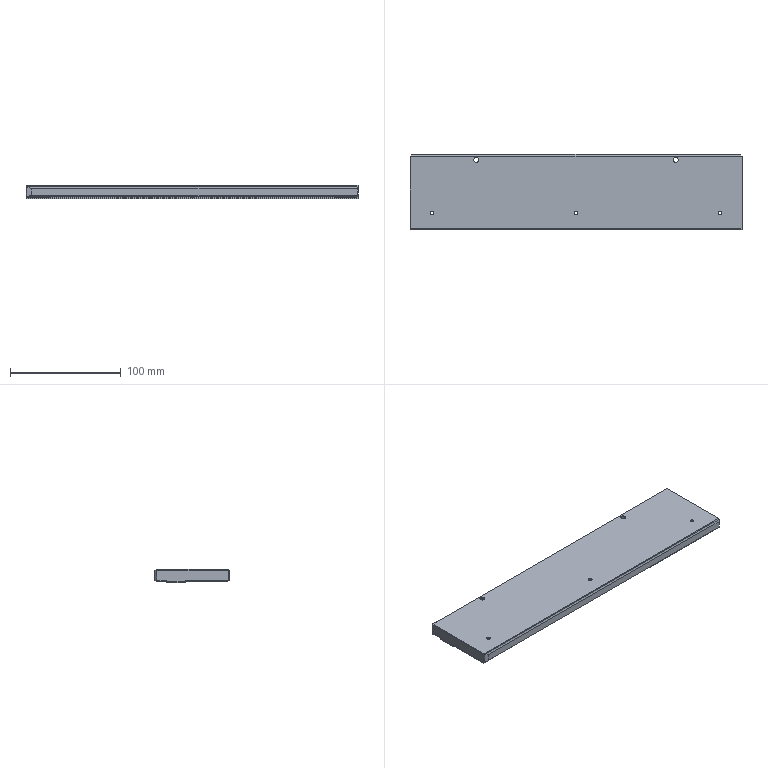Part | 2 solids | 48 faces | box 300 x 68 x 12 mm | volume 409266 mm3 | plane 38 | cylinder 10 | commonest cylinder face diameters 3.242 x6 4.5 x4
STEP:
#1=CARTESIAN_POINT('',(-150.,23.,-6.));
#2=VERTEX_POINT('',#1);
#3=CARTESIAN_POINT('',(150.,23.,-6.));
#4=VERTEX_POINT('',#3);
#5=CARTESIAN_POINT('',(-150.,23.,-6.));
#6=DIRECTION('',(1.,0.,0.));
#7=VECTOR('',#6,1000.);
#8=LINE('',#5,#7);
#9=EDGE_CURVE('',#2,#4,#8,.T.);
#10=ORIENTED_EDGE('',*,*,#9,.T.);
#11=CARTESIAN_POINT('',(150.,6.,-6.));
#12=VERTEX_POINT('',#11);
#13=CARTESIAN_POINT('',(150.,0.,-6.));
#14=DIRECTION('',(0.,-1.,0.));
#15=VECTOR('',#14,1000.);
#16=LINE('',#13,#15);
#17=EDGE_CURVE('',#4,#12,#16,.T.);
#18=ORIENTED_EDGE('',*,*,#17,.T.);
#19=CARTESIAN_POINT('',(-150.,6.,-6.));
#20=VERTEX_POINT('',#19);
#21=CARTESIAN_POINT('',(150.,6.,-6.));
#22=DIRECTION('',(-1.,0.,0.));
#23=VECTOR('',#22,1000.);
#24=LINE('',#21,#23);
#25=EDGE_CURVE('',#12,#20,#24,.T.);
#26=ORIENTED_EDGE('',*,*,#25,.T.);
#27=CARTESIAN_POINT('',(-150.,0.,-6.));
#28=DIRECTION('',(0.,1.,0.));
#29=VECTOR('',#28,1000.);
#30=LINE('',#27,#29);
#31=EDGE_CURVE('',#20,#2,#30,.T.);
#32=ORIENTED_EDGE('',*,*,#31,.T.);
#33=EDGE_LOOP('',(#10,#18,#26,#32));
#34=FACE_BOUND('',#33,.T.);
#35=CARTESIAN_POINT('',(0.,0.,-6.));
#36=DIRECTION('',(0.,0.,-1.));
#37=DIRECTION('',(-1.,0.,0.));
#38=AXIS2_PLACEMENT_3D('',#35,#36,#37);
#39=PLANE('',#38);
#40=ADVANCED_FACE('',(#34),#39,.T.);
#41=CARTESIAN_POINT('',(92.25,29.,6.));
#42=VERTEX_POINT('',#41);
#43=CARTESIAN_POINT('',(90.,29.,6.));
#44=DIRECTION('',(0.,0.,1.));
#45=DIRECTION('',(1.,0.,0.));
#46=AXIS2_PLACEMENT_3D('',#43,#44,#45);
#47=CIRCLE('',#46,2.25);
#48=EDGE_CURVE('',#42,#42,#47,.F.);
#49=ORIENTED_EDGE('',*,*,#48,.F.);
#50=EDGE_LOOP('',(#49));
#51=FACE_BOUND('',#50,.T.);
#52=CARTESIAN_POINT('',(92.25,29.,-4.8));
#53=VERTEX_POINT('',#52);
#54=CARTESIAN_POINT('',(90.,29.,-4.8));
#55=DIRECTION('',(0.,0.,1.));
#56=DIRECTION('',(1.,0.,0.));
#57=AXIS2_PLACEMENT_3D('',#54,#55,#56);
#58=CIRCLE('',#57,2.25);
#59=EDGE_CURVE('',#53,#53,#58,.F.);
#60=ORIENTED_EDGE('',*,*,#59,.T.);
#61=EDGE_LOOP('',(#60));
#62=FACE_BOUND('',#61,.T.);
#63=CARTESIAN_POINT('',(90.,29.,539.357));
#64=DIRECTION('',(0.,0.,-1.));
#65=DIRECTION('',(-1.,0.,0.));
#66=AXIS2_PLACEMENT_3D('',#63,#64,#65);
#67=CYLINDRICAL_SURFACE('',#66,2.25);
#68=ADVANCED_FACE('',(#51,#62),#67,.F.);
#69=CARTESIAN_POINT('',(-87.75,29.,6.));
#70=VERTEX_POINT('',#69);
#71=CARTESIAN_POINT('',(-90.,29.,6.));
#72=DIRECTION('',(0.,0.,1.));
#73=DIRECTION('',(1.,0.,0.));
#74=AXIS2_PLACEMENT_3D('',#71,#72,#73);
#75=CIRCLE('',#74,2.25);
#76=EDGE_CURVE('',#70,#70,#75,.F.);
#77=ORIENTED_EDGE('',*,*,#76,.F.);
#78=EDGE_LOOP('',(#77));
#79=FACE_BOUND('',#78,.T.);
#80=CARTESIAN_POINT('',(-87.75,29.,-4.8));
#81=VERTEX_POINT('',#80);
#82=CARTESIAN_POINT('',(-90.,29.,-4.8));
#83=DIRECTION('',(0.,0.,1.));
#84=DIRECTION('',(1.,0.,0.));
#85=AXIS2_PLACEMENT_3D('',#82,#83,#84);
#86=CIRCLE('',#85,2.25);
#87=EDGE_CURVE('',#81,#81,#86,.F.);
#88=ORIENTED_EDGE('',*,*,#87,.T.);
#89=EDGE_LOOP('',(#88));
#90=FACE_BOUND('',#89,.T.);
#91=CARTESIAN_POINT('',(-90.,29.,539.357));
#92=DIRECTION('',(0.,0.,-1.));
#93=DIRECTION('',(-1.,0.,0.));
#94=AXIS2_PLACEMENT_3D('',#91,#92,#93);
#95=CYLINDRICAL_SURFACE('',#94,2.25);
#96=ADVANCED_FACE('',(#79,#90),#95,.F.);
#97=CARTESIAN_POINT('',(131.621,-19.,-4.8));
#98=VERTEX_POINT('',#97);
#99=CARTESIAN_POINT('',(130.,-19.,-4.8));
#100=DIRECTION('',(0.,0.,1.));
#101=DIRECTION('',(1.,0.,0.));
#102=AXIS2_PLACEMENT_3D('',#99,#100,#101);
#103=CIRCLE('',#102,1.621);
#104=EDGE_CURVE('',#98,#98,#103,.F.);
#105=ORIENTED_EDGE('',*,*,#104,.T.);
#106=EDGE_LOOP('',(#105));
#107=FACE_BOUND('',#106,.T.);
#108=CARTESIAN_POINT('',(131.621,-19.,6.));
#109=VERTEX_POINT('',#108);
#110=CARTESIAN_POINT('',(130.,-19.,6.));
#111=DIRECTION('',(0.,0.,1.));
#112=DIRECTION('',(1.,0.,0.));
#113=AXIS2_PLACEMENT_3D('',#110,#111,#112);
#114=CIRCLE('',#113,1.621);
#115=EDGE_CURVE('',#109,#109,#114,.F.);
#116=ORIENTED_EDGE('',*,*,#115,.F.);
#117=EDGE_LOOP('',(#116));
#118=FACE_BOUND('',#117,.T.);
#119=CARTESIAN_POINT('',(130.,-19.,-302.773));
#120=DIRECTION('',(0.,0.,1.));
#121=DIRECTION('',(1.,0.,0.));
#122=AXIS2_PLACEMENT_3D('',#119,#120,#121);
#123=CYLINDRICAL_SURFACE('',#122,1.621);
#124=ADVANCED_FACE('',(#107,#118),#123,.F.);
#125=CARTESIAN_POINT('',(1.621,-19.,-4.8));
#126=VERTEX_POINT('',#125);
#127=CARTESIAN_POINT('',(0.,-19.,-4.8));
#128=DIRECTION('',(0.,0.,1.));
#129=DIRECTION('',(1.,0.,0.));
#130=AXIS2_PLACEMENT_3D('',#127,#128,#129);
#131=CIRCLE('',#130,1.621);
#132=EDGE_CURVE('',#126,#126,#131,.F.);
#133=ORIENTED_EDGE('',*,*,#132,.T.);
#134=EDGE_LOOP('',(#133));
#135=FACE_BOUND('',#134,.T.);
#136=CARTESIAN_POINT('',(1.621,-19.,6.));
#137=VERTEX_POINT('',#136);
#138=CARTESIAN_POINT('',(0.,-19.,6.));
#139=DIRECTION('',(0.,0.,1.));
#140=DIRECTION('',(1.,0.,0.));
#141=AXIS2_PLACEMENT_3D('',#138,#139,#140);
#142=CIRCLE('',#141,1.621);
#143=EDGE_CURVE('',#137,#137,#142,.F.);
#144=ORIENTED_EDGE('',*,*,#143,.F.);
#145=EDGE_LOOP('',(#144));
#146=FACE_BOUND('',#145,.T.);
#147=CARTESIAN_POINT('',(0.,-19.,-302.773));
#148=DIRECTION('',(0.,0.,1.));
#149=DIRECTION('',(1.,0.,0.));
#150=AXIS2_PLACEMENT_3D('',#147,#148,#149);
#151=CYLINDRICAL_SURFACE('',#150,1.621);
#152=ADVANCED_FACE('',(#135,#146),#151,.F.);
#153=CARTESIAN_POINT('',(-128.379,-19.,-4.8));
#154=VERTEX_POINT('',#153);
#155=CARTESIAN_POINT('',(-130.,-19.,-4.8));
#156=DIRECTION('',(0.,0.,1.));
#157=DIRECTION('',(1.,0.,0.));
#158=AXIS2_PLACEMENT_3D('',#155,#156,#157);
#159=CIRCLE('',#158,1.621);
#160=EDGE_CURVE('',#154,#154,#159,.F.);
#161=ORIENTED_EDGE('',*,*,#160,.T.);
#162=EDGE_LOOP('',(#161));
#163=FACE_BOUND('',#162,.T.);
#164=CARTESIAN_POINT('',(-128.379,-19.,6.));
#165=VERTEX_POINT('',#164);
#166=CARTESIAN_POINT('',(-130.,-19.,6.));
#167=DIRECTION('',(0.,0.,1.));
#168=DIRECTION('',(1.,0.,0.));
#169=AXIS2_PLACEMENT_3D('',#166,#167,#168);
#170=CIRCLE('',#169,1.621);
#171=EDGE_CURVE('',#165,#165,#170,.F.);
#172=ORIENTED_EDGE('',*,*,#171,.F.);
#173=EDGE_LOOP('',(#172));
#174=FACE_BOUND('',#173,.T.);
#175=CARTESIAN_POINT('',(-130.,-19.,-302.773));
#176=DIRECTION('',(0.,0.,1.));
#177=DIRECTION('',(1.,0.,0.));
#178=AXIS2_PLACEMENT_3D('',#175,#176,#177);
#179=CYLINDRICAL_SURFACE('',#178,1.621);
#180=ADVANCED_FACE('',(#163,#174),#179,.F.);
#181=ORIENTED_EDGE('',*,*,#25,.F.);
#182=CARTESIAN_POINT('',(150.,6.,-4.8));
#183=VERTEX_POINT('',#182);
#184=CARTESIAN_POINT('',(150.,6.,-2.5));
#185=DIRECTION('',(0.,0.,-1.));
#186=VECTOR('',#185,1000.);
#187=LINE('',#184,#186);
#188=EDGE_CURVE('',#183,#12,#187,.T.);
#189=ORIENTED_EDGE('',*,*,#188,.F.);
#190=CARTESIAN_POINT('',(-150.,6.,-4.8));
#191=VERTEX_POINT('',#190);
#192=CARTESIAN_POINT('',(0.,6.,-4.8));
#193=DIRECTION('',(-1.,0.,0.));
#194=VECTOR('',#193,1000.);
#195=LINE('',#192,#194);
#196=EDGE_CURVE('',#183,#191,#195,.T.);
#197=ORIENTED_EDGE('',*,*,#196,.T.);
#198=CARTESIAN_POINT('',(-150.,6.,-2.5));
#199=DIRECTION('',(0.,0.,1.));
#200=VECTOR('',#199,1000.);
#201=LINE('',#198,#200);
#202=EDGE_CURVE('',#20,#191,#201,.T.);
#203=ORIENTED_EDGE('',*,*,#202,.F.);
#204=EDGE_LOOP('',(#181,#189,#197,#203));
#205=FACE_BOUND('',#204,.T.);
#206=CARTESIAN_POINT('',(150.,6.,-5.));
#207=DIRECTION('',(0.,1.,0.));
#208=DIRECTION('',(-1.,0.,0.));
#209=AXIS2_PLACEMENT_3D('',#206,#207,#208);
#210=PLANE('',#209);
#211=ADVANCED_FACE('',(#205),#210,.F.);
#212=ORIENTED_EDGE('',*,*,#59,.F.);
#213=EDGE_LOOP('',(#212));
#214=FACE_BOUND('',#213,.T.);
#215=ORIENTED_EDGE('',*,*,#87,.F.);
#216=EDGE_LOOP('',(#215));
#217=FACE_BOUND('',#216,.T.);
#218=CARTESIAN_POINT('',(149.5,32.5,-4.8));
#219=VERTEX_POINT('',#218);
#220=CARTESIAN_POINT('',(-149.5,32.5,-4.8));
#221=VERTEX_POINT('',#220);
#222=CARTESIAN_POINT('',(0.,32.5,-4.8));
#223=DIRECTION('',(-1.,0.,0.));
#224=VECTOR('',#223,1000.);
#225=LINE('',#222,#224);
#226=EDGE_CURVE('',#219,#221,#225,.T.);
#227=ORIENTED_EDGE('',*,*,#226,.F.);
#228=CARTESIAN_POINT('',(150.,32.,-4.8));
#229=VERTEX_POINT('',#228);
#230=CARTESIAN_POINT('',(76.75,105.25,-4.8));
#231=DIRECTION('',(-0.7071,0.7071,0.));
#232=VECTOR('',#231,1000.);
#233=LINE('',#230,#232);
#234=EDGE_CURVE('',#229,#219,#233,.T.);
#235=ORIENTED_EDGE('',*,*,#234,.F.);
#236=CARTESIAN_POINT('',(150.,23.,-4.8));
#237=VERTEX_POINT('',#236);
#238=CARTESIAN_POINT('',(150.,28.5,-4.8));
#239=DIRECTION('',(0.,1.,0.));
#240=VECTOR('',#239,1000.);
#241=LINE('',#238,#240);
#242=EDGE_CURVE('',#237,#229,#241,.T.);
#243=ORIENTED_EDGE('',*,*,#242,.F.);
#244=CARTESIAN_POINT('',(-150.,23.,-4.8));
#245=VERTEX_POINT('',#244);
#246=CARTESIAN_POINT('',(0.,23.,-4.8));
#247=DIRECTION('',(1.,0.,0.));
#248=VECTOR('',#247,1000.);
#249=LINE('',#246,#248);
#250=EDGE_CURVE('',#245,#237,#249,.T.);
#251=ORIENTED_EDGE('',*,*,#250,.F.);
#252=CARTESIAN_POINT('',(-150.,32.,-4.8));
#253=VERTEX_POINT('',#252);
#254=CARTESIAN_POINT('',(-150.,28.5,-4.8));
#255=DIRECTION('',(0.,-1.,0.));
#256=VECTOR('',#255,1000.);
#257=LINE('',#254,#256);
#258=EDGE_CURVE('',#253,#245,#257,.T.);
#259=ORIENTED_EDGE('',*,*,#258,.F.);
#260=CARTESIAN_POINT('',(-76.75,105.25,-4.8));
#261=DIRECTION('',(-0.7071,-0.7071,0.));
#262=VECTOR('',#261,1000.);
#263=LINE('',#260,#262);
#264=EDGE_CURVE('',#221,#253,#263,.T.);
#265=ORIENTED_EDGE('',*,*,#264,.F.);
#266=EDGE_LOOP('',(#227,#235,#243,#251,#259,#265));
#267=FACE_BOUND('',#266,.T.);
#268=CARTESIAN_POINT('',(0.,28.5,-4.8));
#269=DIRECTION('',(0.,0.,1.));
#270=DIRECTION('',(1.,0.,0.));
#271=AXIS2_PLACEMENT_3D('',#268,#269,#270);
#272=PLANE('',#271);
#273=ADVANCED_FACE('',(#214,#217,#267),#272,.F.);
#274=ORIENTED_EDGE('',*,*,#9,.F.);
#275=CARTESIAN_POINT('',(-150.,23.,-2.5));
#276=DIRECTION('',(0.,0.,-1.));
#277=VECTOR('',#276,1000.);
#278=LINE('',#275,#277);
#279=EDGE_CURVE('',#245,#2,#278,.T.);
#280=ORIENTED_EDGE('',*,*,#279,.F.);
#281=ORIENTED_EDGE('',*,*,#250,.T.);
#282=CARTESIAN_POINT('',(150.,23.,-2.5));
#283=DIRECTION('',(0.,0.,1.));
#284=VECTOR('',#283,1000.);
#285=LINE('',#282,#284);
#286=EDGE_CURVE('',#4,#237,#285,.T.);
#287=ORIENTED_EDGE('',*,*,#286,.F.);
#288=EDGE_LOOP('',(#274,#280,#281,#287));
#289=FACE_BOUND('',#288,.T.);
#290=CARTESIAN_POINT('',(-150.,23.,-5.));
#291=DIRECTION('',(0.,-1.,0.));
#292=DIRECTION('',(1.,0.,0.));
#293=AXIS2_PLACEMENT_3D('',#290,#291,#292);
#294=PLANE('',#293);
#295=ADVANCED_FACE('',(#289),#294,.F.);
#296=CARTESIAN_POINT('',(149.5,-34.,3.));
#297=VERTEX_POINT('',#296);
#298=CARTESIAN_POINT('',(149.5,-34.,-3.3));
#299=VERTEX_POINT('',#298);
#300=CARTESIAN_POINT('',(149.5,-34.,0.));
#301=DIRECTION('',(0.,0.,-1.));
#302=VECTOR('',#301,1000.);
#303=LINE('',#300,#302);
#304=EDGE_CURVE('',#297,#299,#303,.T.);
#305=ORIENTED_EDGE('',*,*,#304,.F.);
#306=CARTESIAN_POINT('',(-145.,-34.,3.));
#307=VERTEX_POINT('',#306);
#308=CARTESIAN_POINT('',(-75.,-34.,3.));
#309=DIRECTION('',(1.,0.,0.));
#310=VECTOR('',#309,1000.);
#311=LINE('',#308,#310);
#312=EDGE_CURVE('',#307,#297,#311,.T.);
#313=ORIENTED_EDGE('',*,*,#312,.F.);
#314=CARTESIAN_POINT('',(-145.,-34.,-3.3));
#315=VERTEX_POINT('',#314);
#316=CARTESIAN_POINT('',(-145.,-34.,0.));
#317=DIRECTION('',(0.,0.,1.));
#318=VECTOR('',#317,1000.);
#319=LINE('',#316,#318);
#320=EDGE_CURVE('',#315,#307,#319,.T.);
#321=ORIENTED_EDGE('',*,*,#320,.F.);
#322=CARTESIAN_POINT('',(-75.,-34.,-3.3));
#323=DIRECTION('',(-1.,0.,0.));
#324=VECTOR('',#323,1000.);
#325=LINE('',#322,#324);
#326=EDGE_CURVE('',#299,#315,#325,.T.);
#327=ORIENTED_EDGE('',*,*,#326,.F.);
#328=EDGE_LOOP('',(#305,#313,#321,#327));
#329=FACE_BOUND('',#328,.T.);
#330=CARTESIAN_POINT('',(-150.,-34.,0.));
#331=DIRECTION('',(0.,-1.,0.));
#332=DIRECTION('',(1.,0.,0.));
#333=AXIS2_PLACEMENT_3D('',#330,#331,#332);
#334=PLANE('',#333);
#335=ADVANCED_FACE('',(#329),#334,.T.);
#336=CARTESIAN_POINT('',(-149.502,-33.55,4.801));
#337=VERTEX_POINT('',#336);
#338=CARTESIAN_POINT('',(-149.774,-33.25,6.));
#339=VERTEX_POINT('',#338);
#340=CARTESIAN_POINT('',(-147.229,-36.062,-5.248));
#341=DIRECTION('',(-0.2144,0.2369,0.9476));
#342=VECTOR('',#341,1000.);
#343=LINE('',#340,#342);
#344=EDGE_CURVE('',#337,#339,#343,.T.);
#345=ORIENTED_EDGE('',*,*,#344,.F.);
#346=CARTESIAN_POINT('',(-115.833,-36.917,-8.667));
#347=DIRECTION('',(-0.9245,0.09245,0.3698));
#348=VECTOR('',#347,1000.);
#349=LINE('',#346,#348);
#350=EDGE_CURVE('',#307,#337,#349,.T.);
#351=ORIENTED_EDGE('',*,*,#350,.F.);
#352=ORIENTED_EDGE('',*,*,#312,.T.);
#353=CARTESIAN_POINT('',(150.,-33.5,5.));
#354=VERTEX_POINT('',#353);
#355=CARTESIAN_POINT('',(143.062,-40.438,-22.75));
#356=DIRECTION('',(-0.2357,-0.2357,-0.9428));
#357=VECTOR('',#356,1000.);
#358=LINE('',#355,#357);
#359=EDGE_CURVE('',#354,#297,#358,.T.);
#360=ORIENTED_EDGE('',*,*,#359,.F.);
#361=CARTESIAN_POINT('',(150.,-33.25,6.));
#362=VERTEX_POINT('',#361);
#363=CARTESIAN_POINT('',(150.,-33.75,4.));
#364=DIRECTION('',(0.,0.2425,0.9701));
#365=VECTOR('',#364,1000.);
#366=LINE('',#363,#365);
#367=EDGE_CURVE('',#354,#362,#366,.T.);
#368=ORIENTED_EDGE('',*,*,#367,.T.);
#369=CARTESIAN_POINT('',(-75.,-33.25,6.));
#370=DIRECTION('',(-1.,0.,0.));
#371=VECTOR('',#370,1000.);
#372=LINE('',#369,#371);
#373=EDGE_CURVE('',#362,#339,#372,.T.);
#374=ORIENTED_EDGE('',*,*,#373,.T.);
#375=EDGE_LOOP('',(#345,#351,#352,#360,#368,#374));
#376=FACE_BOUND('',#375,.T.);
#377=CARTESIAN_POINT('',(-75.,-33.75,4.));
#378=DIRECTION('',(0.,-0.9701,0.2425));
#379=DIRECTION('',(0.,-0.2425,-0.9701));
#380=AXIS2_PLACEMENT_3D('',#377,#378,#379);
#381=PLANE('',#380);
#382=ADVANCED_FACE('',(#376),#381,.T.);
#383=CARTESIAN_POINT('',(149.5,32.5,6.));
#384=VERTEX_POINT('',#383);
#385=CARTESIAN_POINT('',(148.,34.,4.5));
#386=VERTEX_POINT('',#385);
#387=CARTESIAN_POINT('',(135.5,46.5,-8.));
#388=DIRECTION('',(-0.5774,0.5774,-0.5774));
#389=VECTOR('',#388,1000.);
#390=LINE('',#387,#389);
#391=EDGE_CURVE('',#384,#386,#390,.T.);
#392=ORIENTED_EDGE('',*,*,#391,.F.);
#393=CARTESIAN_POINT('',(150.,32.,6.));
#394=VERTEX_POINT('',#393);
#395=CARTESIAN_POINT('',(149.,33.,6.));
#396=DIRECTION('',(0.7071,-0.7071,0.));
#397=VECTOR('',#396,1000.);
#398=LINE('',#395,#397);
#399=EDGE_CURVE('',#384,#394,#398,.T.);
#400=ORIENTED_EDGE('',*,*,#399,.T.);
#401=CARTESIAN_POINT('',(150.,32.,0.));
#402=DIRECTION('',(0.,0.,-1.));
#403=VECTOR('',#402,1000.);
#404=LINE('',#401,#403);
#405=EDGE_CURVE('',#394,#229,#404,.T.);
#406=ORIENTED_EDGE('',*,*,#405,.T.);
#407=ORIENTED_EDGE('',*,*,#234,.T.);
#408=CARTESIAN_POINT('',(148.,34.,-3.3));
#409=VERTEX_POINT('',#408);
#410=CARTESIAN_POINT('',(135.7,46.3,9.));
#411=DIRECTION('',(0.5774,-0.5774,-0.5774));
#412=VECTOR('',#411,1000.);
#413=LINE('',#410,#412);
#414=EDGE_CURVE('',#409,#219,#413,.T.);
#415=ORIENTED_EDGE('',*,*,#414,.F.);
#416=CARTESIAN_POINT('',(148.,34.,0.));
#417=DIRECTION('',(0.,0.,1.));
#418=VECTOR('',#417,1000.);
#419=LINE('',#416,#418);
#420=EDGE_CURVE('',#409,#386,#419,.T.);
#421=ORIENTED_EDGE('',*,*,#420,.T.);
#422=EDGE_LOOP('',(#392,#400,#406,#407,#415,#421));
#423=FACE_BOUND('',#422,.T.);
#424=CARTESIAN_POINT('',(149.,33.,0.));
#425=DIRECTION('',(0.7071,0.7071,0.));
#426=DIRECTION('',(0.,0.,-1.));
#427=AXIS2_PLACEMENT_3D('',#424,#425,#426);
#428=PLANE('',#427);
#429=ADVANCED_FACE('',(#423),#428,.T.);
#430=CARTESIAN_POINT('',(-149.502,-33.55,-3.75));
#431=VERTEX_POINT('',#430);
#432=CARTESIAN_POINT('',(-149.502,-33.55,0.));
#433=DIRECTION('',(0.,0.,1.));
#434=VECTOR('',#433,1000.);
#435=LINE('',#432,#434);
#436=EDGE_CURVE('',#431,#337,#435,.T.);
#437=ORIENTED_EDGE('',*,*,#436,.F.);
#438=CARTESIAN_POINT('',(-111.787,-37.321,0.02132));
#439=DIRECTION('',(-0.9901,0.09901,-0.09901));
#440=VECTOR('',#439,1000.);
#441=LINE('',#438,#440);
#442=EDGE_CURVE('',#315,#431,#441,.T.);
#443=ORIENTED_EDGE('',*,*,#442,.F.);
#444=ORIENTED_EDGE('',*,*,#320,.T.);
#445=ORIENTED_EDGE('',*,*,#350,.T.);
#446=EDGE_LOOP('',(#437,#443,#444,#445));
#447=FACE_BOUND('',#446,.T.);
#448=CARTESIAN_POINT('',(-147.5,-33.75,0.));
#449=DIRECTION('',(-0.0995,-0.995,0.));
#450=DIRECTION('',(0.,0.,-1.));
#451=AXIS2_PLACEMENT_3D('',#448,#449,#450);
#452=PLANE('',#451);
#453=ADVANCED_FACE('',(#447),#452,.T.);
#454=CARTESIAN_POINT('',(150.,-33.5,-3.8));
#455=VERTEX_POINT('',#454);
#456=CARTESIAN_POINT('',(150.,-33.5,0.));
#457=DIRECTION('',(0.,0.,1.));
#458=VECTOR('',#457,1000.);
#459=LINE('',#456,#458);
#460=EDGE_CURVE('',#455,#354,#459,.T.);
#461=ORIENTED_EDGE('',*,*,#460,.F.);
#462=CARTESIAN_POINT('',(150.,-32.5,-4.8));
#463=VERTEX_POINT('',#462);
#464=CARTESIAN_POINT('',(150.,-35.65,-1.65));
#465=DIRECTION('',(0.,0.7071,-0.7071));
#466=VECTOR('',#465,1000.);
#467=LINE('',#464,#466);
#468=EDGE_CURVE('',#455,#463,#467,.T.);
#469=ORIENTED_EDGE('',*,*,#468,.T.);
#470=CARTESIAN_POINT('',(150.,28.5,-4.8));
#471=DIRECTION('',(0.,1.,0.));
#472=VECTOR('',#471,1000.);
#473=LINE('',#470,#472);
#474=EDGE_CURVE('',#463,#183,#473,.T.);
#475=ORIENTED_EDGE('',*,*,#474,.T.);
#476=ORIENTED_EDGE('',*,*,#188,.T.);
#477=ORIENTED_EDGE('',*,*,#17,.F.);
#478=ORIENTED_EDGE('',*,*,#286,.T.);
#479=ORIENTED_EDGE('',*,*,#242,.T.);
#480=ORIENTED_EDGE('',*,*,#405,.F.);
#481=CARTESIAN_POINT('',(150.,0.,6.));
#482=DIRECTION('',(0.,1.,0.));
#483=VECTOR('',#482,1000.);
#484=LINE('',#481,#483);
#485=EDGE_CURVE('',#362,#394,#484,.T.);
#486=ORIENTED_EDGE('',*,*,#485,.F.);
#487=ORIENTED_EDGE('',*,*,#367,.F.);
#488=EDGE_LOOP('',(#461,#469,#475,#476,#477,#478,#479,#480,#486,#487));
#489=FACE_BOUND('',#488,.T.);
#490=CARTESIAN_POINT('',(150.,-34.,0.));
#491=DIRECTION('',(1.,0.,0.));
#492=DIRECTION('',(0.,1.,0.));
#493=AXIS2_PLACEMENT_3D('',#490,#491,#492);
#494=PLANE('',#493);
#495=ADVANCED_FACE('',(#489),#494,.T.);
#496=CARTESIAN_POINT('',(-150.,-33.,-4.3));
#497=VERTEX_POINT('',#496);
#498=CARTESIAN_POINT('',(-138.094,-46.156,8.856));
#499=DIRECTION('',(0.539,-0.5956,0.5956));
#500=VECTOR('',#499,1000.);
#501=LINE('',#498,#500);
#502=EDGE_CURVE('',#497,#431,#501,.T.);
#503=ORIENTED_EDGE('',*,*,#502,.F.);
#504=CARTESIAN_POINT('',(-150.,-32.5,-4.8));
#505=VERTEX_POINT('',#504);
#506=CARTESIAN_POINT('',(-150.,-33.75,-3.55));
#507=DIRECTION('',(0.,0.7071,-0.7071));
#508=VECTOR('',#507,1000.);
#509=LINE('',#506,#508);
#510=EDGE_CURVE('',#497,#505,#509,.T.);
#511=ORIENTED_EDGE('',*,*,#510,.T.);
#512=CARTESIAN_POINT('',(0.,-32.5,-4.8));
#513=DIRECTION('',(1.,0.,0.));
#514=VECTOR('',#513,1000.);
#515=LINE('',#512,#514);
#516=EDGE_CURVE('',#505,#463,#515,.T.);
#517=ORIENTED_EDGE('',*,*,#516,.T.);
#518=ORIENTED_EDGE('',*,*,#468,.F.);
#519=CARTESIAN_POINT('',(149.5,-34.,-3.3));
#520=DIRECTION('',(0.5774,0.5774,-0.5774));
#521=VECTOR('',#520,1000.);
#522=LINE('',#519,#521);
#523=EDGE_CURVE('',#299,#455,#522,.T.);
#524=ORIENTED_EDGE('',*,*,#523,.F.);
#525=ORIENTED_EDGE('',*,*,#326,.T.);
#526=ORIENTED_EDGE('',*,*,#442,.T.);
#527=EDGE_LOOP('',(#503,#511,#517,#518,#524,#525,#526));
#528=FACE_BOUND('',#527,.T.);
#529=CARTESIAN_POINT('',(-75.,-33.75,-3.55));
#530=DIRECTION('',(0.,-0.7071,-0.7071));
#531=DIRECTION('',(-1.,0.,0.));
#532=AXIS2_PLACEMENT_3D('',#529,#530,#531);
#533=PLANE('',#532);
#534=ADVANCED_FACE('',(#528),#533,.T.);
#535=ORIENTED_EDGE('',*,*,#460,.T.);
#536=ORIENTED_EDGE('',*,*,#359,.T.);
#537=ORIENTED_EDGE('',*,*,#304,.T.);
#538=ORIENTED_EDGE('',*,*,#523,.T.);
#539=EDGE_LOOP('',(#535,#536,#537,#538));
#540=FACE_BOUND('',#539,.T.);
#541=CARTESIAN_POINT('',(149.75,-33.75,0.));
#542=DIRECTION('',(0.7071,-0.7071,0.));
#543=DIRECTION('',(0.,0.,-1.));
#544=AXIS2_PLACEMENT_3D('',#541,#542,#543);
#545=PLANE('',#544);
#546=ADVANCED_FACE('',(#540),#545,.T.);
#547=CARTESIAN_POINT('',(-148.,34.,-3.3));
#548=VERTEX_POINT('',#547);
#549=CARTESIAN_POINT('',(-110.7,71.3,34.));
#550=DIRECTION('',(0.5774,0.5774,0.5774));
#551=VECTOR('',#550,1000.);
#552=LINE('',#549,#551);
#553=EDGE_CURVE('',#221,#548,#552,.T.);
#554=ORIENTED_EDGE('',*,*,#553,.T.);
#555=CARTESIAN_POINT('',(75.,34.,-3.3));
#556=DIRECTION('',(1.,0.,0.));
#557=VECTOR('',#556,1000.);
#558=LINE('',#555,#557);
#559=EDGE_CURVE('',#548,#409,#558,.T.);
#560=ORIENTED_EDGE('',*,*,#559,.T.);
#561=ORIENTED_EDGE('',*,*,#414,.T.);
#562=ORIENTED_EDGE('',*,*,#226,.T.);
#563=EDGE_LOOP('',(#554,#560,#561,#562));
#564=FACE_BOUND('',#563,.T.);
#565=CARTESIAN_POINT('',(75.,33.75,-3.55));
#566=DIRECTION('',(0.,0.7071,-0.7071));
#567=DIRECTION('',(-1.,0.,0.));
#568=AXIS2_PLACEMENT_3D('',#565,#566,#567);
#569=PLANE('',#568);
#570=ADVANCED_FACE('',(#564),#569,.T.);
#571=CARTESIAN_POINT('',(-148.,34.,4.5));
#572=VERTEX_POINT('',#571);
#573=CARTESIAN_POINT('',(75.,34.,4.5));
#574=DIRECTION('',(-1.,0.,0.));
#575=VECTOR('',#574,1000.);
#576=LINE('',#573,#575);
#577=EDGE_CURVE('',#386,#572,#576,.T.);
#578=ORIENTED_EDGE('',*,*,#577,.F.);
#579=ORIENTED_EDGE('',*,*,#420,.F.);
#580=ORIENTED_EDGE('',*,*,#559,.F.);
#581=CARTESIAN_POINT('',(-148.,34.,0.));
#582=DIRECTION('',(0.,0.,-1.));
#583=VECTOR('',#582,1000.);
#584=LINE('',#581,#583);
#585=EDGE_CURVE('',#572,#548,#584,.T.);
#586=ORIENTED_EDGE('',*,*,#585,.F.);
#587=EDGE_LOOP('',(#578,#579,#580,#586));
#588=FACE_BOUND('',#587,.T.);
#589=CARTESIAN_POINT('',(150.,34.,0.));
#590=DIRECTION('',(0.,1.,0.));
#591=DIRECTION('',(-1.,0.,0.));
#592=AXIS2_PLACEMENT_3D('',#589,#590,#591);
#593=PLANE('',#592);
#594=ADVANCED_FACE('',(#588),#593,.T.);
#595=CARTESIAN_POINT('',(-149.5,32.5,6.));
#596=VERTEX_POINT('',#595);
#597=CARTESIAN_POINT('',(-110.5,71.5,-33.));
#598=DIRECTION('',(-0.5774,-0.5774,0.5774));
#599=VECTOR('',#598,1000.);
#600=LINE('',#597,#599);
#601=EDGE_CURVE('',#572,#596,#600,.T.);
#602=ORIENTED_EDGE('',*,*,#601,.F.);
#603=ORIENTED_EDGE('',*,*,#585,.T.);
#604=ORIENTED_EDGE('',*,*,#553,.F.);
#605=ORIENTED_EDGE('',*,*,#264,.T.);
#606=CARTESIAN_POINT('',(-150.,32.,6.));
#607=VERTEX_POINT('',#606);
#608=CARTESIAN_POINT('',(-150.,32.,0.));
#609=DIRECTION('',(0.,0.,1.));
#610=VECTOR('',#609,1000.);
#611=LINE('',#608,#610);
#612=EDGE_CURVE('',#253,#607,#611,.T.);
#613=ORIENTED_EDGE('',*,*,#612,.T.);
#614=CARTESIAN_POINT('',(-149.,33.,6.));
#615=DIRECTION('',(0.7071,0.7071,0.));
#616=VECTOR('',#615,1000.);
#617=LINE('',#614,#616);
#618=EDGE_CURVE('',#607,#596,#617,.T.);
#619=ORIENTED_EDGE('',*,*,#618,.T.);
#620=EDGE_LOOP('',(#602,#603,#604,#605,#613,#619));
#621=FACE_BOUND('',#620,.T.);
#622=CARTESIAN_POINT('',(-149.,33.,0.));
#623=DIRECTION('',(-0.7071,0.7071,0.));
#624=DIRECTION('',(0.,0.,1.));
#625=AXIS2_PLACEMENT_3D('',#622,#623,#624);
#626=PLANE('',#625);
#627=ADVANCED_FACE('',(#621),#626,.T.);
#628=ORIENTED_EDGE('',*,*,#601,.T.);
#629=CARTESIAN_POINT('',(75.,32.5,6.));
#630=DIRECTION('',(1.,0.,0.));
#631=VECTOR('',#630,1000.);
#632=LINE('',#629,#631);
#633=EDGE_CURVE('',#596,#384,#632,.T.);
#634=ORIENTED_EDGE('',*,*,#633,.T.);
#635=ORIENTED_EDGE('',*,*,#391,.T.);
#636=ORIENTED_EDGE('',*,*,#577,.T.);
#637=EDGE_LOOP('',(#628,#634,#635,#636));
#638=FACE_BOUND('',#637,.T.);
#639=CARTESIAN_POINT('',(75.,33.75,4.75));
#640=DIRECTION('',(0.,0.7071,0.7071));
#641=DIRECTION('',(1.,0.,0.));
#642=AXIS2_PLACEMENT_3D('',#639,#640,#641);
#643=PLANE('',#642);
#644=ADVANCED_FACE('',(#638),#643,.T.);
#645=ORIENTED_EDGE('',*,*,#171,.T.);
#646=EDGE_LOOP('',(#645));
#647=FACE_BOUND('',#646,.T.);
#648=ORIENTED_EDGE('',*,*,#143,.T.);
#649=EDGE_LOOP('',(#648));
#650=FACE_BOUND('',#649,.T.);
#651=ORIENTED_EDGE('',*,*,#115,.T.);
#652=EDGE_LOOP('',(#651));
#653=FACE_BOUND('',#652,.T.);
#654=ORIENTED_EDGE('',*,*,#76,.T.);
#655=EDGE_LOOP('',(#654));
#656=FACE_BOUND('',#655,.T.);
#657=ORIENTED_EDGE('',*,*,#48,.T.);
#658=EDGE_LOOP('',(#657));
#659=FACE_BOUND('',#658,.T.);
#660=CARTESIAN_POINT('',(-150.,-33.,6.));
#661=VERTEX_POINT('',#660);
#662=CARTESIAN_POINT('',(-149.751,-33.275,6.));
#663=DIRECTION('',(-0.671,0.7415,0.));
#664=VECTOR('',#663,1000.);
#665=LINE('',#662,#664);
#666=EDGE_CURVE('',#339,#661,#665,.T.);
#667=ORIENTED_EDGE('',*,*,#666,.F.);
#668=ORIENTED_EDGE('',*,*,#373,.F.);
#669=ORIENTED_EDGE('',*,*,#485,.T.);
#670=ORIENTED_EDGE('',*,*,#399,.F.);
#671=ORIENTED_EDGE('',*,*,#633,.F.);
#672=ORIENTED_EDGE('',*,*,#618,.F.);
#673=CARTESIAN_POINT('',(-150.,0.,6.));
#674=DIRECTION('',(0.,-1.,0.));
#675=VECTOR('',#674,1000.);
#676=LINE('',#673,#675);
#677=EDGE_CURVE('',#607,#661,#676,.T.);
#678=ORIENTED_EDGE('',*,*,#677,.T.);
#679=EDGE_LOOP('',(#667,#668,#669,#670,#671,#672,#678));
#680=FACE_BOUND('',#679,.T.);
#681=CARTESIAN_POINT('',(0.,0.,6.));
#682=DIRECTION('',(0.,0.,1.));
#683=DIRECTION('',(1.,0.,0.));
#684=AXIS2_PLACEMENT_3D('',#681,#682,#683);
#685=PLANE('',#684);
#686=ADVANCED_FACE('',(#647,#650,#653,#656,#659,#680),#685,.T.);
#687=ORIENTED_EDGE('',*,*,#510,.F.);
#688=CARTESIAN_POINT('',(-150.,-33.,0.));
#689=DIRECTION('',(0.,0.,-1.));
#690=VECTOR('',#689,1000.);
#691=LINE('',#688,#690);
#692=EDGE_CURVE('',#661,#497,#691,.T.);
#693=ORIENTED_EDGE('',*,*,#692,.F.);
#694=ORIENTED_EDGE('',*,*,#677,.F.);
#695=ORIENTED_EDGE('',*,*,#612,.F.);
#696=ORIENTED_EDGE('',*,*,#258,.T.);
#697=ORIENTED_EDGE('',*,*,#279,.T.);
#698=ORIENTED_EDGE('',*,*,#31,.F.);
#699=ORIENTED_EDGE('',*,*,#202,.T.);
#700=CARTESIAN_POINT('',(-150.,28.5,-4.8));
#701=DIRECTION('',(0.,-1.,0.));
#702=VECTOR('',#701,1000.);
#703=LINE('',#700,#702);
#704=EDGE_CURVE('',#191,#505,#703,.T.);
#705=ORIENTED_EDGE('',*,*,#704,.T.);
#706=EDGE_LOOP('',(#687,#693,#694,#695,#696,#697,#698,#699,#705));
#707=FACE_BOUND('',#706,.T.);
#708=CARTESIAN_POINT('',(-150.,34.,0.));
#709=DIRECTION('',(-1.,0.,0.));
#710=DIRECTION('',(0.,-1.,0.));
#711=AXIS2_PLACEMENT_3D('',#708,#709,#710);
#712=PLANE('',#711);
#713=ADVANCED_FACE('',(#707),#712,.T.);
#714=ORIENTED_EDGE('',*,*,#104,.F.);
#715=EDGE_LOOP('',(#714));
#716=FACE_BOUND('',#715,.T.);
#717=ORIENTED_EDGE('',*,*,#132,.F.);
#718=EDGE_LOOP('',(#717));
#719=FACE_BOUND('',#718,.T.);
#720=ORIENTED_EDGE('',*,*,#160,.F.);
#721=EDGE_LOOP('',(#720));
#722=FACE_BOUND('',#721,.T.);
#723=ORIENTED_EDGE('',*,*,#516,.F.);
#724=ORIENTED_EDGE('',*,*,#704,.F.);
#725=ORIENTED_EDGE('',*,*,#196,.F.);
#726=ORIENTED_EDGE('',*,*,#474,.F.);
#727=EDGE_LOOP('',(#723,#724,#725,#726));
#728=FACE_BOUND('',#727,.T.);
#729=CARTESIAN_POINT('',(0.,28.5,-4.8));
#730=DIRECTION('',(0.,0.,1.));
#731=DIRECTION('',(1.,0.,0.));
#732=AXIS2_PLACEMENT_3D('',#729,#730,#731);
#733=PLANE('',#732);
#734=ADVANCED_FACE('',(#716,#719,#722,#728),#733,.F.);
#735=ORIENTED_EDGE('',*,*,#692,.T.);
#736=ORIENTED_EDGE('',*,*,#502,.T.);
#737=ORIENTED_EDGE('',*,*,#436,.T.);
#738=ORIENTED_EDGE('',*,*,#344,.T.);
#739=ORIENTED_EDGE('',*,*,#666,.T.);
#740=EDGE_LOOP('',(#735,#736,#737,#738,#739));
#741=FACE_BOUND('',#740,.T.);
#742=CARTESIAN_POINT('',(-149.751,-33.275,0.));
#743=DIRECTION('',(-0.7415,-0.671,0.));
#744=DIRECTION('',(0.,0.,1.));
#745=AXIS2_PLACEMENT_3D('',#742,#743,#744);
#746=PLANE('',#745);
#747=ADVANCED_FACE('',(#741),#746,.T.);
#748=CLOSED_SHELL('',(#40,#68,#96,#124,#152,#180,#211,#273,#295,#335,#382,#429,#453,#495,#534,#546,#570,#594,#627,#644,#686,#713,#734,#747));
#749=MANIFOLD_SOLID_BREP('',#748);
#750=CARTESIAN_POINT('',(-150.,23.,-5.));
#751=VERTEX_POINT('',#750);
#752=CARTESIAN_POINT('',(150.,23.,-5.));
#753=VERTEX_POINT('',#752);
#754=CARTESIAN_POINT('',(-75.,23.,-5.));
#755=DIRECTION('',(1.,0.,0.));
#756=VECTOR('',#755,1000.);
#757=LINE('',#754,#756);
#758=EDGE_CURVE('',#751,#753,#757,.T.);
#759=ORIENTED_EDGE('',*,*,#758,.T.);
#760=CARTESIAN_POINT('',(150.,6.,-5.));
#761=VERTEX_POINT('',#760);
#762=CARTESIAN_POINT('',(150.,-34.,-5.));
#763=DIRECTION('',(0.,-1.,0.));
#764=VECTOR('',#763,1000.);
#765=LINE('',#762,#764);
#766=EDGE_CURVE('',#753,#761,#765,.T.);
#767=ORIENTED_EDGE('',*,*,#766,.T.);
#768=CARTESIAN_POINT('',(-150.,6.,-5.));
#769=VERTEX_POINT('',#768);
#770=CARTESIAN_POINT('',(75.,6.,-5.));
#771=DIRECTION('',(-1.,0.,0.));
#772=VECTOR('',#771,1000.);
#773=LINE('',#770,#772);
#774=EDGE_CURVE('',#761,#769,#773,.T.);
#775=ORIENTED_EDGE('',*,*,#774,.T.);
#776=CARTESIAN_POINT('',(-150.,34.,-5.));
#777=DIRECTION('',(0.,1.,0.));
#778=VECTOR('',#777,1000.);
#779=LINE('',#776,#778);
#780=EDGE_CURVE('',#769,#751,#779,.T.);
#781=ORIENTED_EDGE('',*,*,#780,.T.);
#782=EDGE_LOOP('',(#759,#767,#775,#781));
#783=FACE_BOUND('',#782,.T.);
#784=CARTESIAN_POINT('',(0.,0.,-5.));
#785=DIRECTION('',(0.,0.,-1.));
#786=DIRECTION('',(-1.,0.,0.));
#787=AXIS2_PLACEMENT_3D('',#784,#785,#786);
#788=PLANE('',#787);
#789=ADVANCED_FACE('',(#783),#788,.T.);
#790=CARTESIAN_POINT('',(87.75,29.,5.));
#791=VERTEX_POINT('',#790);
#792=CARTESIAN_POINT('',(90.,29.,5.));
#793=DIRECTION('',(0.,0.,-1.));
#794=DIRECTION('',(-1.,0.,0.));
#795=AXIS2_PLACEMENT_3D('',#792,#793,#794);
#796=CIRCLE('',#795,2.25);
#797=EDGE_CURVE('',#791,#791,#796,.T.);
#798=ORIENTED_EDGE('',*,*,#797,.F.);
#799=EDGE_LOOP('',(#798));
#800=FACE_BOUND('',#799,.T.);
#801=CARTESIAN_POINT('',(87.75,29.,-3.8));
#802=VERTEX_POINT('',#801);
#803=CARTESIAN_POINT('',(90.,29.,-3.8));
#804=DIRECTION('',(0.,0.,-1.));
#805=DIRECTION('',(-1.,0.,0.));
#806=AXIS2_PLACEMENT_3D('',#803,#804,#805);
#807=CIRCLE('',#806,2.25);
#808=EDGE_CURVE('',#802,#802,#807,.T.);
#809=ORIENTED_EDGE('',*,*,#808,.T.);
#810=EDGE_LOOP('',(#809));
#811=FACE_BOUND('',#810,.T.);
#812=CARTESIAN_POINT('',(90.,29.,539.357));
#813=DIRECTION('',(0.,0.,-1.));
#814=DIRECTION('',(-1.,0.,0.));
#815=AXIS2_PLACEMENT_3D('',#812,#813,#814);
#816=CYLINDRICAL_SURFACE('',#815,2.25);
#817=ADVANCED_FACE('',(#800,#811),#816,.F.);
#818=CARTESIAN_POINT('',(-92.25,29.,5.));
#819=VERTEX_POINT('',#818);
#820=CARTESIAN_POINT('',(-90.,29.,5.));
#821=DIRECTION('',(0.,0.,-1.));
#822=DIRECTION('',(-1.,0.,0.));
#823=AXIS2_PLACEMENT_3D('',#820,#821,#822);
#824=CIRCLE('',#823,2.25);
#825=EDGE_CURVE('',#819,#819,#824,.T.);
#826=ORIENTED_EDGE('',*,*,#825,.F.);
#827=EDGE_LOOP('',(#826));
#828=FACE_BOUND('',#827,.T.);
#829=CARTESIAN_POINT('',(-92.25,29.,-3.8));
#830=VERTEX_POINT('',#829);
#831=CARTESIAN_POINT('',(-90.,29.,-3.8));
#832=DIRECTION('',(0.,0.,-1.));
#833=DIRECTION('',(-1.,0.,0.));
#834=AXIS2_PLACEMENT_3D('',#831,#832,#833);
#835=CIRCLE('',#834,2.25);
#836=EDGE_CURVE('',#830,#830,#835,.T.);
#837=ORIENTED_EDGE('',*,*,#836,.T.);
#838=EDGE_LOOP('',(#837));
#839=FACE_BOUND('',#838,.T.);
#840=CARTESIAN_POINT('',(-90.,29.,539.357));
#841=DIRECTION('',(0.,0.,-1.));
#842=DIRECTION('',(-1.,0.,0.));
#843=AXIS2_PLACEMENT_3D('',#840,#841,#842);
#844=CYLINDRICAL_SURFACE('',#843,2.25);
#845=ADVANCED_FACE('',(#828,#839),#844,.F.);
#846=CARTESIAN_POINT('',(131.621,-19.,-3.8));
#847=VERTEX_POINT('',#846);
#848=CARTESIAN_POINT('',(130.,-19.,-3.8));
#849=DIRECTION('',(0.,0.,-1.));
#850=DIRECTION('',(1.,0.,0.));
#851=AXIS2_PLACEMENT_3D('',#848,#849,#850);
#852=CIRCLE('',#851,1.621);
#853=EDGE_CURVE('',#847,#847,#852,.T.);
#854=ORIENTED_EDGE('',*,*,#853,.T.);
#855=EDGE_LOOP('',(#854));
#856=FACE_BOUND('',#855,.T.);
#857=CARTESIAN_POINT('',(131.621,-19.,5.));
#858=VERTEX_POINT('',#857);
#859=CARTESIAN_POINT('',(130.,-19.,5.));
#860=DIRECTION('',(0.,0.,-1.));
#861=DIRECTION('',(1.,0.,0.));
#862=AXIS2_PLACEMENT_3D('',#859,#860,#861);
#863=CIRCLE('',#862,1.621);
#864=EDGE_CURVE('',#858,#858,#863,.T.);
#865=ORIENTED_EDGE('',*,*,#864,.F.);
#866=EDGE_LOOP('',(#865));
#867=FACE_BOUND('',#866,.T.);
#868=CARTESIAN_POINT('',(130.,-19.,-302.773));
#869=DIRECTION('',(0.,0.,1.));
#870=DIRECTION('',(1.,0.,0.));
#871=AXIS2_PLACEMENT_3D('',#868,#869,#870);
#872=CYLINDRICAL_SURFACE('',#871,1.621);
#873=ADVANCED_FACE('',(#856,#867),#872,.F.);
#874=CARTESIAN_POINT('',(1.621,-19.,-3.8));
#875=VERTEX_POINT('',#874);
#876=CARTESIAN_POINT('',(0.,-19.,-3.8));
#877=DIRECTION('',(0.,0.,-1.));
#878=DIRECTION('',(1.,0.,0.));
#879=AXIS2_PLACEMENT_3D('',#876,#877,#878);
#880=CIRCLE('',#879,1.621);
#881=EDGE_CURVE('',#875,#875,#880,.T.);
#882=ORIENTED_EDGE('',*,*,#881,.T.);
#883=EDGE_LOOP('',(#882));
#884=FACE_BOUND('',#883,.T.);
#885=CARTESIAN_POINT('',(1.621,-19.,5.));
#886=VERTEX_POINT('',#885);
#887=CARTESIAN_POINT('',(0.,-19.,5.));
#888=DIRECTION('',(0.,0.,-1.));
#889=DIRECTION('',(1.,0.,0.));
#890=AXIS2_PLACEMENT_3D('',#887,#888,#889);
#891=CIRCLE('',#890,1.621);
#892=EDGE_CURVE('',#886,#886,#891,.T.);
#893=ORIENTED_EDGE('',*,*,#892,.F.);
#894=EDGE_LOOP('',(#893));
#895=FACE_BOUND('',#894,.T.);
#896=CARTESIAN_POINT('',(0.,-19.,-302.773));
#897=DIRECTION('',(0.,0.,1.));
#898=DIRECTION('',(1.,0.,0.));
#899=AXIS2_PLACEMENT_3D('',#896,#897,#898);
#900=CYLINDRICAL_SURFACE('',#899,1.621);
#901=ADVANCED_FACE('',(#884,#895),#900,.F.);
#902=CARTESIAN_POINT('',(-128.379,-19.,-3.8));
#903=VERTEX_POINT('',#902);
#904=CARTESIAN_POINT('',(-130.,-19.,-3.8));
#905=DIRECTION('',(0.,0.,-1.));
#906=DIRECTION('',(1.,0.,0.));
#907=AXIS2_PLACEMENT_3D('',#904,#905,#906);
#908=CIRCLE('',#907,1.621);
#909=EDGE_CURVE('',#903,#903,#908,.T.);
#910=ORIENTED_EDGE('',*,*,#909,.T.);
#911=EDGE_LOOP('',(#910));
#912=FACE_BOUND('',#911,.T.);
#913=CARTESIAN_POINT('',(-128.379,-19.,5.));
#914=VERTEX_POINT('',#913);
#915=CARTESIAN_POINT('',(-130.,-19.,5.));
#916=DIRECTION('',(0.,0.,-1.));
#917=DIRECTION('',(1.,0.,0.));
#918=AXIS2_PLACEMENT_3D('',#915,#916,#917);
#919=CIRCLE('',#918,1.621);
#920=EDGE_CURVE('',#914,#914,#919,.T.);
#921=ORIENTED_EDGE('',*,*,#920,.F.);
#922=EDGE_LOOP('',(#921));
#923=FACE_BOUND('',#922,.T.);
#924=CARTESIAN_POINT('',(-130.,-19.,-302.773));
#925=DIRECTION('',(0.,0.,1.));
#926=DIRECTION('',(1.,0.,0.));
#927=AXIS2_PLACEMENT_3D('',#924,#925,#926);
#928=CYLINDRICAL_SURFACE('',#927,1.621);
#929=ADVANCED_FACE('',(#912,#923),#928,.F.);
#930=ORIENTED_EDGE('',*,*,#774,.F.);
#931=CARTESIAN_POINT('',(150.,6.,-3.8));
#932=VERTEX_POINT('',#931);
#933=CARTESIAN_POINT('',(150.,6.,-2.5));
#934=DIRECTION('',(0.,0.,-1.));
#935=VECTOR('',#934,1000.);
#936=LINE('',#933,#935);
#937=EDGE_CURVE('',#932,#761,#936,.T.);
#938=ORIENTED_EDGE('',*,*,#937,.F.);
#939=CARTESIAN_POINT('',(-150.,6.,-3.8));
#940=VERTEX_POINT('',#939);
#941=CARTESIAN_POINT('',(150.,6.,-3.8));
#942=DIRECTION('',(-1.,0.,0.));
#943=VECTOR('',#942,1000.);
#944=LINE('',#941,#943);
#945=EDGE_CURVE('',#932,#940,#944,.T.);
#946=ORIENTED_EDGE('',*,*,#945,.T.);
#947=CARTESIAN_POINT('',(-150.,6.,-2.5));
#948=DIRECTION('',(0.,0.,1.));
#949=VECTOR('',#948,1000.);
#950=LINE('',#947,#949);
#951=EDGE_CURVE('',#769,#940,#950,.T.);
#952=ORIENTED_EDGE('',*,*,#951,.F.);
#953=EDGE_LOOP('',(#930,#938,#946,#952));
#954=FACE_BOUND('',#953,.T.);
#955=CARTESIAN_POINT('',(150.,6.,-5.));
#956=DIRECTION('',(0.,1.,0.));
#957=DIRECTION('',(-1.,0.,0.));
#958=AXIS2_PLACEMENT_3D('',#955,#956,#957);
#959=PLANE('',#958);
#960=ADVANCED_FACE('',(#954),#959,.F.);
#961=ORIENTED_EDGE('',*,*,#808,.F.);
#962=EDGE_LOOP('',(#961));
#963=FACE_BOUND('',#962,.T.);
#964=ORIENTED_EDGE('',*,*,#836,.F.);
#965=EDGE_LOOP('',(#964));
#966=FACE_BOUND('',#965,.T.);
#967=CARTESIAN_POINT('',(148.5,33.5,-3.8));
#968=VERTEX_POINT('',#967);
#969=CARTESIAN_POINT('',(-148.5,33.5,-3.8));
#970=VERTEX_POINT('',#969);
#971=CARTESIAN_POINT('',(75.,33.5,-3.8));
#972=DIRECTION('',(-1.,0.,0.));
#973=VECTOR('',#972,1000.);
#974=LINE('',#971,#973);
#975=EDGE_CURVE('',#968,#970,#974,.T.);
#976=ORIENTED_EDGE('',*,*,#975,.F.);
#977=CARTESIAN_POINT('',(150.,32.,-3.8));
#978=VERTEX_POINT('',#977);
#979=CARTESIAN_POINT('',(112.875,69.125,-3.8));
#980=DIRECTION('',(-0.7071,0.7071,0.));
#981=VECTOR('',#980,1000.);
#982=LINE('',#979,#981);
#983=EDGE_CURVE('',#978,#968,#982,.T.);
#984=ORIENTED_EDGE('',*,*,#983,.F.);
#985=CARTESIAN_POINT('',(150.,23.,-3.8));
#986=VERTEX_POINT('',#985);
#987=CARTESIAN_POINT('',(150.,-2.75,-3.8));
#988=DIRECTION('',(0.,1.,0.));
#989=VECTOR('',#988,1000.);
#990=LINE('',#987,#989);
#991=EDGE_CURVE('',#986,#978,#990,.T.);
#992=ORIENTED_EDGE('',*,*,#991,.F.);
#993=CARTESIAN_POINT('',(-150.,23.,-3.8));
#994=VERTEX_POINT('',#993);
#995=CARTESIAN_POINT('',(150.,23.,-3.8));
#996=DIRECTION('',(1.,0.,0.));
#997=VECTOR('',#996,1000.);
#998=LINE('',#995,#997);
#999=EDGE_CURVE('',#994,#986,#998,.T.);
#1000=ORIENTED_EDGE('',*,*,#999,.F.);
#1001=CARTESIAN_POINT('',(-150.,32.,-3.8));
#1002=VERTEX_POINT('',#1001);
#1003=CARTESIAN_POINT('',(-150.,31.25,-3.8));
#1004=DIRECTION('',(0.,-1.,0.));
#1005=VECTOR('',#1004,1000.);
#1006=LINE('',#1003,#1005);
#1007=EDGE_CURVE('',#1002,#994,#1006,.T.);
#1008=ORIENTED_EDGE('',*,*,#1007,.F.);
#1009=CARTESIAN_POINT('',(-112.875,69.125,-3.8));
#1010=DIRECTION('',(-0.7071,-0.7071,0.));
#1011=VECTOR('',#1010,1000.);
#1012=LINE('',#1009,#1011);
#1013=EDGE_CURVE('',#970,#1002,#1012,.T.);
#1014=ORIENTED_EDGE('',*,*,#1013,.F.);
#1015=EDGE_LOOP('',(#976,#984,#992,#1000,#1008,#1014));
#1016=FACE_BOUND('',#1015,.T.);
#1017=CARTESIAN_POINT('',(0.,28.5,-3.8));
#1018=DIRECTION('',(0.,0.,1.));
#1019=DIRECTION('',(1.,0.,0.));
#1020=AXIS2_PLACEMENT_3D('',#1017,#1018,#1019);
#1021=PLANE('',#1020);
#1022=ADVANCED_FACE('',(#963,#966,#1016),#1021,.F.);
#1023=ORIENTED_EDGE('',*,*,#758,.F.);
#1024=CARTESIAN_POINT('',(-150.,23.,-2.5));
#1025=DIRECTION('',(0.,0.,-1.));
#1026=VECTOR('',#1025,1000.);
#1027=LINE('',#1024,#1026);
#1028=EDGE_CURVE('',#994,#751,#1027,.T.);
#1029=ORIENTED_EDGE('',*,*,#1028,.F.);
#1030=ORIENTED_EDGE('',*,*,#999,.T.);
#1031=CARTESIAN_POINT('',(150.,23.,-2.5));
#1032=DIRECTION('',(0.,0.,1.));
#1033=VECTOR('',#1032,1000.);
#1034=LINE('',#1031,#1033);
#1035=EDGE_CURVE('',#753,#986,#1034,.T.);
#1036=ORIENTED_EDGE('',*,*,#1035,.F.);
#1037=EDGE_LOOP('',(#1023,#1029,#1030,#1036));
#1038=FACE_BOUND('',#1037,.T.);
#1039=CARTESIAN_POINT('',(-150.,23.,-5.));
#1040=DIRECTION('',(0.,-1.,0.));
#1041=DIRECTION('',(1.,0.,0.));
#1042=AXIS2_PLACEMENT_3D('',#1039,#1040,#1041);
#1043=PLANE('',#1042);
#1044=ADVANCED_FACE('',(#1038),#1043,.F.);
#1045=CARTESIAN_POINT('',(149.5,-34.,3.));
#1046=VERTEX_POINT('',#1045);
#1047=CARTESIAN_POINT('',(149.5,-34.,-3.3));
#1048=VERTEX_POINT('',#1047);
#1049=CARTESIAN_POINT('',(149.5,-34.,0.));
#1050=DIRECTION('',(0.,0.,-1.));
#1051=VECTOR('',#1050,1000.);
#1052=LINE('',#1049,#1051);
#1053=EDGE_CURVE('',#1046,#1048,#1052,.T.);
#1054=ORIENTED_EDGE('',*,*,#1053,.F.);
#1055=CARTESIAN_POINT('',(-145.,-34.,3.));
#1056=VERTEX_POINT('',#1055);
#1057=CARTESIAN_POINT('',(-75.,-34.,3.));
#1058=DIRECTION('',(1.,0.,0.));
#1059=VECTOR('',#1058,1000.);
#1060=LINE('',#1057,#1059);
#1061=EDGE_CURVE('',#1056,#1046,#1060,.T.);
#1062=ORIENTED_EDGE('',*,*,#1061,.F.);
#1063=CARTESIAN_POINT('',(-145.,-34.,-3.3));
#1064=VERTEX_POINT('',#1063);
#1065=CARTESIAN_POINT('',(-145.,-34.,0.));
#1066=DIRECTION('',(0.,0.,1.));
#1067=VECTOR('',#1066,1000.);
#1068=LINE('',#1065,#1067);
#1069=EDGE_CURVE('',#1064,#1056,#1068,.T.);
#1070=ORIENTED_EDGE('',*,*,#1069,.F.);
#1071=CARTESIAN_POINT('',(-75.,-34.,-3.3));
#1072=DIRECTION('',(-1.,0.,0.));
#1073=VECTOR('',#1072,1000.);
#1074=LINE('',#1071,#1073);
#1075=EDGE_CURVE('',#1048,#1064,#1074,.T.);
#1076=ORIENTED_EDGE('',*,*,#1075,.F.);
#1077=EDGE_LOOP('',(#1054,#1062,#1070,#1076));
#1078=FACE_BOUND('',#1077,.T.);
#1079=CARTESIAN_POINT('',(-150.,-34.,0.));
#1080=DIRECTION('',(0.,-1.,0.));
#1081=DIRECTION('',(1.,0.,0.));
#1082=AXIS2_PLACEMENT_3D('',#1079,#1080,#1081);
#1083=PLANE('',#1082);
#1084=ADVANCED_FACE('',(#1078),#1083,.T.);
#1085=CARTESIAN_POINT('',(-149.502,-33.55,4.801));
#1086=VERTEX_POINT('',#1085);
#1087=CARTESIAN_POINT('',(-149.548,-33.5,5.));
#1088=VERTEX_POINT('',#1087);
#1089=CARTESIAN_POINT('',(-147.229,-36.062,-5.248));
#1090=DIRECTION('',(-0.2144,0.2369,0.9476));
#1091=VECTOR('',#1090,1000.);
#1092=LINE('',#1089,#1091);
#1093=EDGE_CURVE('',#1086,#1088,#1092,.T.);
#1094=ORIENTED_EDGE('',*,*,#1093,.F.);
#1095=CARTESIAN_POINT('',(-115.833,-36.917,-8.667));
#1096=DIRECTION('',(-0.9245,0.09245,0.3698));
#1097=VECTOR('',#1096,1000.);
#1098=LINE('',#1095,#1097);
#1099=EDGE_CURVE('',#1056,#1086,#1098,.T.);
#1100=ORIENTED_EDGE('',*,*,#1099,.F.);
#1101=ORIENTED_EDGE('',*,*,#1061,.T.);
#1102=CARTESIAN_POINT('',(150.,-33.5,5.));
#1103=VERTEX_POINT('',#1102);
#1104=CARTESIAN_POINT('',(143.062,-40.438,-22.75));
#1105=DIRECTION('',(-0.2357,-0.2357,-0.9428));
#1106=VECTOR('',#1105,1000.);
#1107=LINE('',#1104,#1106);
#1108=EDGE_CURVE('',#1103,#1046,#1107,.T.);
#1109=ORIENTED_EDGE('',*,*,#1108,.F.);
#1110=CARTESIAN_POINT('',(-75.,-33.5,5.));
#1111=DIRECTION('',(-1.,0.,0.));
#1112=VECTOR('',#1111,1000.);
#1113=LINE('',#1110,#1112);
#1114=EDGE_CURVE('',#1103,#1088,#1113,.T.);
#1115=ORIENTED_EDGE('',*,*,#1114,.T.);
#1116=EDGE_LOOP('',(#1094,#1100,#1101,#1109,#1115));
#1117=FACE_BOUND('',#1116,.T.);
#1118=CARTESIAN_POINT('',(-75.,-33.75,4.));
#1119=DIRECTION('',(0.,-0.9701,0.2425));
#1120=DIRECTION('',(0.,-0.2425,-0.9701));
#1121=AXIS2_PLACEMENT_3D('',#1118,#1119,#1120);
#1122=PLANE('',#1121);
#1123=ADVANCED_FACE('',(#1117),#1122,.T.);
#1124=CARTESIAN_POINT('',(148.5,33.5,5.));
#1125=VERTEX_POINT('',#1124);
#1126=CARTESIAN_POINT('',(148.,34.,4.5));
#1127=VERTEX_POINT('',#1126);
#1128=CARTESIAN_POINT('',(135.5,46.5,-8.));
#1129=DIRECTION('',(-0.5774,0.5774,-0.5774));
#1130=VECTOR('',#1129,1000.);
#1131=LINE('',#1128,#1130);
#1132=EDGE_CURVE('',#1125,#1127,#1131,.T.);
#1133=ORIENTED_EDGE('',*,*,#1132,.F.);
#1134=CARTESIAN_POINT('',(150.,32.,5.));
#1135=VERTEX_POINT('',#1134);
#1136=CARTESIAN_POINT('',(120.,62.,5.));
#1137=DIRECTION('',(0.7071,-0.7071,0.));
#1138=VECTOR('',#1137,1000.);
#1139=LINE('',#1136,#1138);
#1140=EDGE_CURVE('',#1125,#1135,#1139,.T.);
#1141=ORIENTED_EDGE('',*,*,#1140,.T.);
#1142=CARTESIAN_POINT('',(150.,32.,0.));
#1143=DIRECTION('',(0.,0.,-1.));
#1144=VECTOR('',#1143,1000.);
#1145=LINE('',#1142,#1144);
#1146=EDGE_CURVE('',#1135,#978,#1145,.T.);
#1147=ORIENTED_EDGE('',*,*,#1146,.T.);
#1148=ORIENTED_EDGE('',*,*,#983,.T.);
#1149=CARTESIAN_POINT('',(148.,34.,-3.3));
#1150=VERTEX_POINT('',#1149);
#1151=CARTESIAN_POINT('',(135.7,46.3,9.));
#1152=DIRECTION('',(0.5774,-0.5774,-0.5774));
#1153=VECTOR('',#1152,1000.);
#1154=LINE('',#1151,#1153);
#1155=EDGE_CURVE('',#1150,#968,#1154,.T.);
#1156=ORIENTED_EDGE('',*,*,#1155,.F.);
#1157=CARTESIAN_POINT('',(148.,34.,0.));
#1158=DIRECTION('',(0.,0.,1.));
#1159=VECTOR('',#1158,1000.);
#1160=LINE('',#1157,#1159);
#1161=EDGE_CURVE('',#1150,#1127,#1160,.T.);
#1162=ORIENTED_EDGE('',*,*,#1161,.T.);
#1163=EDGE_LOOP('',(#1133,#1141,#1147,#1148,#1156,#1162));
#1164=FACE_BOUND('',#1163,.T.);
#1165=CARTESIAN_POINT('',(149.,33.,0.));
#1166=DIRECTION('',(0.7071,0.7071,0.));
#1167=DIRECTION('',(0.,0.,-1.));
#1168=AXIS2_PLACEMENT_3D('',#1165,#1166,#1167);
#1169=PLANE('',#1168);
#1170=ADVANCED_FACE('',(#1164),#1169,.T.);
#1171=CARTESIAN_POINT('',(-149.502,-33.55,-3.75));
#1172=VERTEX_POINT('',#1171);
#1173=CARTESIAN_POINT('',(-149.502,-33.55,0.));
#1174=DIRECTION('',(0.,0.,1.));
#1175=VECTOR('',#1174,1000.);
#1176=LINE('',#1173,#1175);
#1177=EDGE_CURVE('',#1172,#1086,#1176,.T.);
#1178=ORIENTED_EDGE('',*,*,#1177,.F.);
#1179=CARTESIAN_POINT('',(-111.787,-37.321,0.02132));
#1180=DIRECTION('',(-0.9901,0.09901,-0.09901));
#1181=VECTOR('',#1180,1000.);
#1182=LINE('',#1179,#1181);
#1183=EDGE_CURVE('',#1064,#1172,#1182,.T.);
#1184=ORIENTED_EDGE('',*,*,#1183,.F.);
#1185=ORIENTED_EDGE('',*,*,#1069,.T.);
#1186=ORIENTED_EDGE('',*,*,#1099,.T.);
#1187=EDGE_LOOP('',(#1178,#1184,#1185,#1186));
#1188=FACE_BOUND('',#1187,.T.);
#1189=CARTESIAN_POINT('',(-147.5,-33.75,0.));
#1190=DIRECTION('',(-0.0995,-0.995,0.));
#1191=DIRECTION('',(0.,0.,-1.));
#1192=AXIS2_PLACEMENT_3D('',#1189,#1190,#1191);
#1193=PLANE('',#1192);
#1194=ADVANCED_FACE('',(#1188),#1193,.T.);
#1195=CARTESIAN_POINT('',(150.,-33.5,-3.8));
#1196=VERTEX_POINT('',#1195);
#1197=CARTESIAN_POINT('',(150.,-33.5,0.));
#1198=DIRECTION('',(0.,0.,1.));
#1199=VECTOR('',#1198,1000.);
#1200=LINE('',#1197,#1199);
#1201=EDGE_CURVE('',#1196,#1103,#1200,.T.);
#1202=ORIENTED_EDGE('',*,*,#1201,.F.);
#1203=CARTESIAN_POINT('',(150.,-34.,-3.8));
#1204=DIRECTION('',(0.,1.,0.));
#1205=VECTOR('',#1204,1000.);
#1206=LINE('',#1203,#1205);
#1207=EDGE_CURVE('',#1196,#932,#1206,.T.);
#1208=ORIENTED_EDGE('',*,*,#1207,.T.);
#1209=ORIENTED_EDGE('',*,*,#937,.T.);
#1210=ORIENTED_EDGE('',*,*,#766,.F.);
#1211=ORIENTED_EDGE('',*,*,#1035,.T.);
#1212=ORIENTED_EDGE('',*,*,#991,.T.);
#1213=ORIENTED_EDGE('',*,*,#1146,.F.);
#1214=CARTESIAN_POINT('',(150.,-34.,5.));
#1215=DIRECTION('',(0.,1.,0.));
#1216=VECTOR('',#1215,1000.);
#1217=LINE('',#1214,#1216);
#1218=EDGE_CURVE('',#1103,#1135,#1217,.T.);
#1219=ORIENTED_EDGE('',*,*,#1218,.F.);
#1220=EDGE_LOOP('',(#1202,#1208,#1209,#1210,#1211,#1212,#1213,#1219));
#1221=FACE_BOUND('',#1220,.T.);
#1222=CARTESIAN_POINT('',(150.,-34.,0.));
#1223=DIRECTION('',(1.,0.,0.));
#1224=DIRECTION('',(0.,1.,0.));
#1225=AXIS2_PLACEMENT_3D('',#1222,#1223,#1224);
#1226=PLANE('',#1225);
#1227=ADVANCED_FACE('',(#1221),#1226,.T.);
#1228=CARTESIAN_POINT('',(-149.548,-33.5,-3.8));
#1229=VERTEX_POINT('',#1228);
#1230=CARTESIAN_POINT('',(-138.094,-46.156,8.856));
#1231=DIRECTION('',(0.539,-0.5956,0.5956));
#1232=VECTOR('',#1231,1000.);
#1233=LINE('',#1230,#1232);
#1234=EDGE_CURVE('',#1229,#1172,#1233,.T.);
#1235=ORIENTED_EDGE('',*,*,#1234,.F.);
#1236=CARTESIAN_POINT('',(-75.,-33.5,-3.8));
#1237=DIRECTION('',(1.,0.,0.));
#1238=VECTOR('',#1237,1000.);
#1239=LINE('',#1236,#1238);
#1240=EDGE_CURVE('',#1229,#1196,#1239,.T.);
#1241=ORIENTED_EDGE('',*,*,#1240,.T.);
#1242=CARTESIAN_POINT('',(149.5,-34.,-3.3));
#1243=DIRECTION('',(0.5774,0.5774,-0.5774));
#1244=VECTOR('',#1243,1000.);
#1245=LINE('',#1242,#1244);
#1246=EDGE_CURVE('',#1048,#1196,#1245,.T.);
#1247=ORIENTED_EDGE('',*,*,#1246,.F.);
#1248=ORIENTED_EDGE('',*,*,#1075,.T.);
#1249=ORIENTED_EDGE('',*,*,#1183,.T.);
#1250=EDGE_LOOP('',(#1235,#1241,#1247,#1248,#1249));
#1251=FACE_BOUND('',#1250,.T.);
#1252=CARTESIAN_POINT('',(-75.,-33.75,-3.55));
#1253=DIRECTION('',(0.,-0.7071,-0.7071));
#1254=DIRECTION('',(-1.,0.,0.));
#1255=AXIS2_PLACEMENT_3D('',#1252,#1253,#1254);
#1256=PLANE('',#1255);
#1257=ADVANCED_FACE('',(#1251),#1256,.T.);
#1258=ORIENTED_EDGE('',*,*,#1201,.T.);
#1259=ORIENTED_EDGE('',*,*,#1108,.T.);
#1260=ORIENTED_EDGE('',*,*,#1053,.T.);
#1261=ORIENTED_EDGE('',*,*,#1246,.T.);
#1262=EDGE_LOOP('',(#1258,#1259,#1260,#1261));
#1263=FACE_BOUND('',#1262,.T.);
#1264=CARTESIAN_POINT('',(149.75,-33.75,0.));
#1265=DIRECTION('',(0.7071,-0.7071,0.));
#1266=DIRECTION('',(0.,0.,-1.));
#1267=AXIS2_PLACEMENT_3D('',#1264,#1265,#1266);
#1268=PLANE('',#1267);
#1269=ADVANCED_FACE('',(#1263),#1268,.T.);
#1270=CARTESIAN_POINT('',(-148.,34.,-3.3));
#1271=VERTEX_POINT('',#1270);
#1272=CARTESIAN_POINT('',(-110.7,71.3,34.));
#1273=DIRECTION('',(0.5774,0.5774,0.5774));
#1274=VECTOR('',#1273,1000.);
#1275=LINE('',#1272,#1274);
#1276=EDGE_CURVE('',#970,#1271,#1275,.T.);
#1277=ORIENTED_EDGE('',*,*,#1276,.T.);
#1278=CARTESIAN_POINT('',(75.,34.,-3.3));
#1279=DIRECTION('',(1.,0.,0.));
#1280=VECTOR('',#1279,1000.);
#1281=LINE('',#1278,#1280);
#1282=EDGE_CURVE('',#1271,#1150,#1281,.T.);
#1283=ORIENTED_EDGE('',*,*,#1282,.T.);
#1284=ORIENTED_EDGE('',*,*,#1155,.T.);
#1285=ORIENTED_EDGE('',*,*,#975,.T.);
#1286=EDGE_LOOP('',(#1277,#1283,#1284,#1285));
#1287=FACE_BOUND('',#1286,.T.);
#1288=CARTESIAN_POINT('',(75.,33.75,-3.55));
#1289=DIRECTION('',(0.,0.7071,-0.7071));
#1290=DIRECTION('',(-1.,0.,0.));
#1291=AXIS2_PLACEMENT_3D('',#1288,#1289,#1290);
#1292=PLANE('',#1291);
#1293=ADVANCED_FACE('',(#1287),#1292,.T.);
#1294=CARTESIAN_POINT('',(-148.,34.,4.5));
#1295=VERTEX_POINT('',#1294);
#1296=CARTESIAN_POINT('',(75.,34.,4.5));
#1297=DIRECTION('',(-1.,0.,0.));
#1298=VECTOR('',#1297,1000.);
#1299=LINE('',#1296,#1298);
#1300=EDGE_CURVE('',#1127,#1295,#1299,.T.);
#1301=ORIENTED_EDGE('',*,*,#1300,.F.);
#1302=ORIENTED_EDGE('',*,*,#1161,.F.);
#1303=ORIENTED_EDGE('',*,*,#1282,.F.);
#1304=CARTESIAN_POINT('',(-148.,34.,0.));
#1305=DIRECTION('',(0.,0.,-1.));
#1306=VECTOR('',#1305,1000.);
#1307=LINE('',#1304,#1306);
#1308=EDGE_CURVE('',#1295,#1271,#1307,.T.);
#1309=ORIENTED_EDGE('',*,*,#1308,.F.);
#1310=EDGE_LOOP('',(#1301,#1302,#1303,#1309));
#1311=FACE_BOUND('',#1310,.T.);
#1312=CARTESIAN_POINT('',(150.,34.,0.));
#1313=DIRECTION('',(0.,1.,0.));
#1314=DIRECTION('',(-1.,0.,0.));
#1315=AXIS2_PLACEMENT_3D('',#1312,#1313,#1314);
#1316=PLANE('',#1315);
#1317=ADVANCED_FACE('',(#1311),#1316,.T.);
#1318=CARTESIAN_POINT('',(-148.5,33.5,5.));
#1319=VERTEX_POINT('',#1318);
#1320=CARTESIAN_POINT('',(-110.5,71.5,-33.));
#1321=DIRECTION('',(-0.5774,-0.5774,0.5774));
#1322=VECTOR('',#1321,1000.);
#1323=LINE('',#1320,#1322);
#1324=EDGE_CURVE('',#1295,#1319,#1323,.T.);
#1325=ORIENTED_EDGE('',*,*,#1324,.F.);
#1326=ORIENTED_EDGE('',*,*,#1308,.T.);
#1327=ORIENTED_EDGE('',*,*,#1276,.F.);
#1328=ORIENTED_EDGE('',*,*,#1013,.T.);
#1329=CARTESIAN_POINT('',(-150.,32.,5.));
#1330=VERTEX_POINT('',#1329);
#1331=CARTESIAN_POINT('',(-150.,32.,0.));
#1332=DIRECTION('',(0.,0.,1.));
#1333=VECTOR('',#1332,1000.);
#1334=LINE('',#1331,#1333);
#1335=EDGE_CURVE('',#1002,#1330,#1334,.T.);
#1336=ORIENTED_EDGE('',*,*,#1335,.T.);
#1337=CARTESIAN_POINT('',(-120.,62.,5.));
#1338=DIRECTION('',(0.7071,0.7071,0.));
#1339=VECTOR('',#1338,1000.);
#1340=LINE('',#1337,#1339);
#1341=EDGE_CURVE('',#1330,#1319,#1340,.T.);
#1342=ORIENTED_EDGE('',*,*,#1341,.T.);
#1343=EDGE_LOOP('',(#1325,#1326,#1327,#1328,#1336,#1342));
#1344=FACE_BOUND('',#1343,.T.);
#1345=CARTESIAN_POINT('',(-149.,33.,0.));
#1346=DIRECTION('',(-0.7071,0.7071,0.));
#1347=DIRECTION('',(0.,0.,1.));
#1348=AXIS2_PLACEMENT_3D('',#1345,#1346,#1347);
#1349=PLANE('',#1348);
#1350=ADVANCED_FACE('',(#1344),#1349,.T.);
#1351=ORIENTED_EDGE('',*,*,#1324,.T.);
#1352=CARTESIAN_POINT('',(75.,33.5,5.));
#1353=DIRECTION('',(1.,0.,0.));
#1354=VECTOR('',#1353,1000.);
#1355=LINE('',#1352,#1354);
#1356=EDGE_CURVE('',#1319,#1125,#1355,.T.);
#1357=ORIENTED_EDGE('',*,*,#1356,.T.);
#1358=ORIENTED_EDGE('',*,*,#1132,.T.);
#1359=ORIENTED_EDGE('',*,*,#1300,.T.);
#1360=EDGE_LOOP('',(#1351,#1357,#1358,#1359));
#1361=FACE_BOUND('',#1360,.T.);
#1362=CARTESIAN_POINT('',(75.,33.75,4.75));
#1363=DIRECTION('',(0.,0.7071,0.7071));
#1364=DIRECTION('',(1.,0.,0.));
#1365=AXIS2_PLACEMENT_3D('',#1362,#1363,#1364);
#1366=PLANE('',#1365);
#1367=ADVANCED_FACE('',(#1361),#1366,.T.);
#1368=ORIENTED_EDGE('',*,*,#920,.T.);
#1369=EDGE_LOOP('',(#1368));
#1370=FACE_BOUND('',#1369,.T.);
#1371=ORIENTED_EDGE('',*,*,#892,.T.);
#1372=EDGE_LOOP('',(#1371));
#1373=FACE_BOUND('',#1372,.T.);
#1374=ORIENTED_EDGE('',*,*,#864,.T.);
#1375=EDGE_LOOP('',(#1374));
#1376=FACE_BOUND('',#1375,.T.);
#1377=ORIENTED_EDGE('',*,*,#825,.T.);
#1378=EDGE_LOOP('',(#1377));
#1379=FACE_BOUND('',#1378,.T.);
#1380=ORIENTED_EDGE('',*,*,#797,.T.);
#1381=EDGE_LOOP('',(#1380));
#1382=FACE_BOUND('',#1381,.T.);
#1383=CARTESIAN_POINT('',(-150.,-33.,5.));
#1384=VERTEX_POINT('',#1383);
#1385=CARTESIAN_POINT('',(-124.316,-61.38,5.));
#1386=DIRECTION('',(-0.671,0.7415,0.));
#1387=VECTOR('',#1386,1000.);
#1388=LINE('',#1385,#1387);
#1389=EDGE_CURVE('',#1088,#1384,#1388,.T.);
#1390=ORIENTED_EDGE('',*,*,#1389,.F.);
#1391=ORIENTED_EDGE('',*,*,#1114,.F.);
#1392=ORIENTED_EDGE('',*,*,#1218,.T.);
#1393=ORIENTED_EDGE('',*,*,#1140,.F.);
#1394=ORIENTED_EDGE('',*,*,#1356,.F.);
#1395=ORIENTED_EDGE('',*,*,#1341,.F.);
#1396=CARTESIAN_POINT('',(-150.,34.,5.));
#1397=DIRECTION('',(0.,-1.,0.));
#1398=VECTOR('',#1397,1000.);
#1399=LINE('',#1396,#1398);
#1400=EDGE_CURVE('',#1330,#1384,#1399,.T.);
#1401=ORIENTED_EDGE('',*,*,#1400,.T.);
#1402=EDGE_LOOP('',(#1390,#1391,#1392,#1393,#1394,#1395,#1401));
#1403=FACE_BOUND('',#1402,.T.);
#1404=CARTESIAN_POINT('',(0.,0.,5.));
#1405=DIRECTION('',(0.,0.,1.));
#1406=DIRECTION('',(1.,0.,0.));
#1407=AXIS2_PLACEMENT_3D('',#1404,#1405,#1406);
#1408=PLANE('',#1407);
#1409=ADVANCED_FACE('',(#1370,#1373,#1376,#1379,#1382,#1403),#1408,.T.);
#1410=CARTESIAN_POINT('',(-150.,-33.,-3.8));
#1411=VERTEX_POINT('',#1410);
#1412=CARTESIAN_POINT('',(-150.,-33.,0.));
#1413=DIRECTION('',(0.,0.,-1.));
#1414=VECTOR('',#1413,1000.);
#1415=LINE('',#1412,#1414);
#1416=EDGE_CURVE('',#1384,#1411,#1415,.T.);
#1417=ORIENTED_EDGE('',*,*,#1416,.F.);
#1418=ORIENTED_EDGE('',*,*,#1400,.F.);
#1419=ORIENTED_EDGE('',*,*,#1335,.F.);
#1420=ORIENTED_EDGE('',*,*,#1007,.T.);
#1421=ORIENTED_EDGE('',*,*,#1028,.T.);
#1422=ORIENTED_EDGE('',*,*,#780,.F.);
#1423=ORIENTED_EDGE('',*,*,#951,.T.);
#1424=CARTESIAN_POINT('',(-150.,34.,-3.8));
#1425=DIRECTION('',(0.,-1.,0.));
#1426=VECTOR('',#1425,1000.);
#1427=LINE('',#1424,#1426);
#1428=EDGE_CURVE('',#940,#1411,#1427,.T.);
#1429=ORIENTED_EDGE('',*,*,#1428,.T.);
#1430=EDGE_LOOP('',(#1417,#1418,#1419,#1420,#1421,#1422,#1423,#1429));
#1431=FACE_BOUND('',#1430,.T.);
#1432=CARTESIAN_POINT('',(-150.,34.,0.));
#1433=DIRECTION('',(-1.,0.,0.));
#1434=DIRECTION('',(0.,-1.,0.));
#1435=AXIS2_PLACEMENT_3D('',#1432,#1433,#1434);
#1436=PLANE('',#1435);
#1437=ADVANCED_FACE('',(#1431),#1436,.T.);
#1438=ORIENTED_EDGE('',*,*,#853,.F.);
#1439=EDGE_LOOP('',(#1438));
#1440=FACE_BOUND('',#1439,.T.);
#1441=ORIENTED_EDGE('',*,*,#881,.F.);
#1442=EDGE_LOOP('',(#1441));
#1443=FACE_BOUND('',#1442,.T.);
#1444=ORIENTED_EDGE('',*,*,#909,.F.);
#1445=EDGE_LOOP('',(#1444));
#1446=FACE_BOUND('',#1445,.T.);
#1447=CARTESIAN_POINT('',(-149.751,-33.275,-3.8));
#1448=DIRECTION('',(0.671,-0.7415,0.));
#1449=VECTOR('',#1448,1000.);
#1450=LINE('',#1447,#1449);
#1451=EDGE_CURVE('',#1411,#1229,#1450,.T.);
#1452=ORIENTED_EDGE('',*,*,#1451,.F.);
#1453=ORIENTED_EDGE('',*,*,#1428,.F.);
#1454=ORIENTED_EDGE('',*,*,#945,.F.);
#1455=ORIENTED_EDGE('',*,*,#1207,.F.);
#1456=ORIENTED_EDGE('',*,*,#1240,.F.);
#1457=EDGE_LOOP('',(#1452,#1453,#1454,#1455,#1456));
#1458=FACE_BOUND('',#1457,.T.);
#1459=CARTESIAN_POINT('',(0.,28.5,-3.8));
#1460=DIRECTION('',(0.,0.,1.));
#1461=DIRECTION('',(1.,0.,0.));
#1462=AXIS2_PLACEMENT_3D('',#1459,#1460,#1461);
#1463=PLANE('',#1462);
#1464=ADVANCED_FACE('',(#1440,#1443,#1446,#1458),#1463,.F.);
#1465=ORIENTED_EDGE('',*,*,#1234,.T.);
#1466=ORIENTED_EDGE('',*,*,#1177,.T.);
#1467=ORIENTED_EDGE('',*,*,#1093,.T.);
#1468=ORIENTED_EDGE('',*,*,#1389,.T.);
#1469=ORIENTED_EDGE('',*,*,#1416,.T.);
#1470=ORIENTED_EDGE('',*,*,#1451,.T.);
#1471=EDGE_LOOP('',(#1465,#1466,#1467,#1468,#1469,#1470));
#1472=FACE_BOUND('',#1471,.T.);
#1473=CARTESIAN_POINT('',(-149.751,-33.275,0.));
#1474=DIRECTION('',(-0.7415,-0.671,0.));
#1475=DIRECTION('',(0.,0.,1.));
#1476=AXIS2_PLACEMENT_3D('',#1473,#1474,#1475);
#1477=PLANE('',#1476);
#1478=ADVANCED_FACE('',(#1472),#1477,.T.);
#1479=CLOSED_SHELL('',(#789,#817,#845,#873,#901,#929,#960,#1022,#1044,#1084,#1123,#1170,#1194,#1227,#1257,#1269,#1293,#1317,#1350,#1367,#1409,#1437,#1464,#1478));
#1480=MANIFOLD_SOLID_BREP('',#1479);
#1481=(LENGTH_UNIT()NAMED_UNIT(*)SI_UNIT(.MILLI.,.METRE.));
#1482=UNCERTAINTY_MEASURE_WITH_UNIT(LENGTH_MEASURE(0.00001),#1481,'','');
#1483=(NAMED_UNIT(*)PLANE_ANGLE_UNIT()SI_UNIT($,.RADIAN.));
#1484=(NAMED_UNIT(*)SI_UNIT($,.STERADIAN.)SOLID_ANGLE_UNIT());
#1485=(GEOMETRIC_REPRESENTATION_CONTEXT(3)GLOBAL_UNCERTAINTY_ASSIGNED_CONTEXT((#1482))GLOBAL_UNIT_ASSIGNED_CONTEXT((#1481,#1483,#1484))REPRESENTATION_CONTEXT('',''));
#1486=ADVANCED_BREP_SHAPE_REPRESENTATION('',(#749,#1480),#1485);